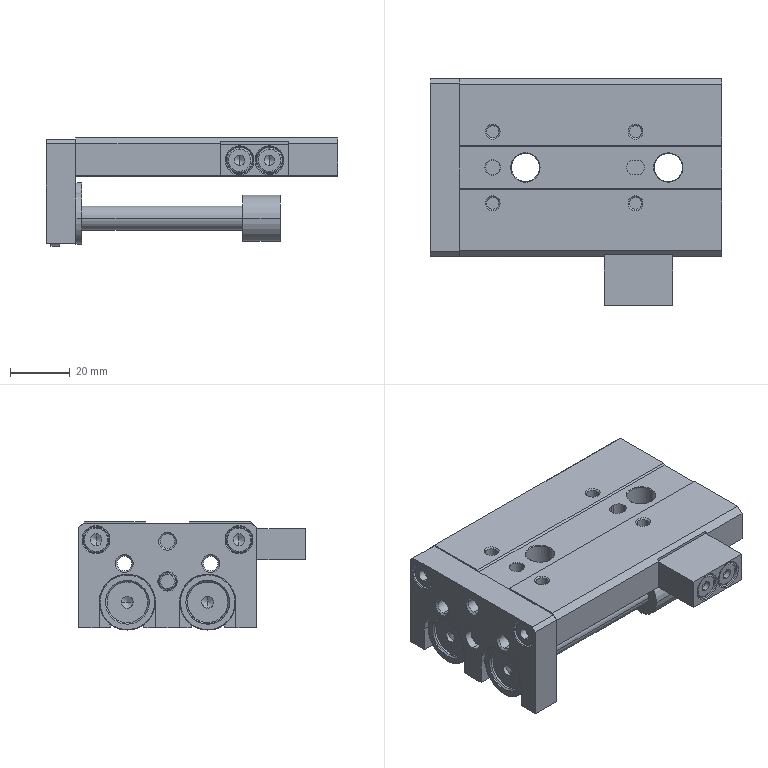Part | SolidWorks | features BaseBody 1 | 1 solid | 287 faces | box 98 x 76.35 x 36.35 mm | volume 83829 mm3 | plane 124 | cylinder 99 | cone 54 | spline 10 | commonest cylinder face diameters 4.134 x12 9 x12 4 x8 8.5 x8 4.917 x6 19.6 x6